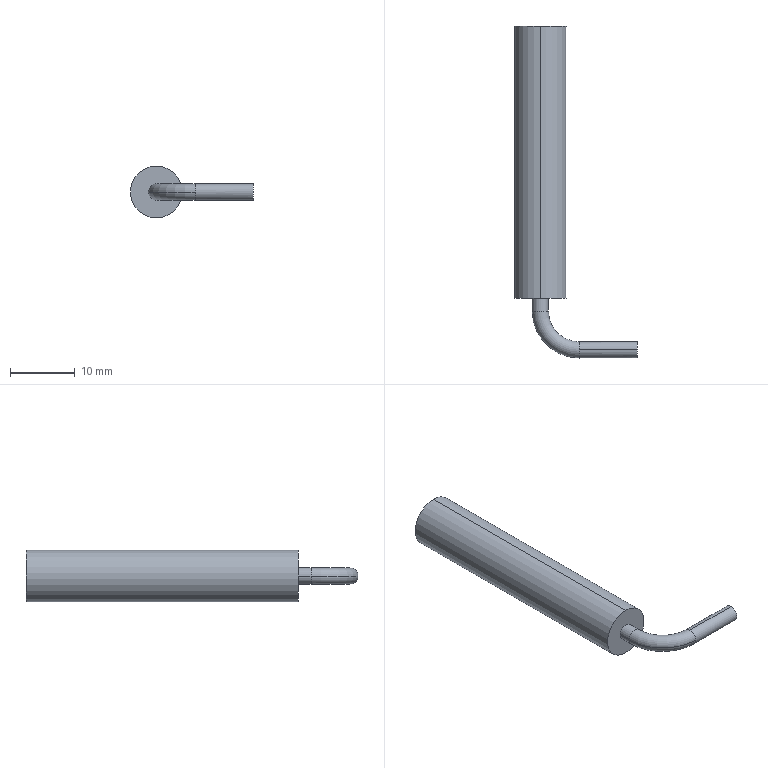Part | SolidWorks | features Extrusion 1, PLine 1, Sweep 1 | 1 solid | 12 faces | box 19 x 51.25 x 8 mm | volume 2211 mm3 | cylinder 6 | plane 4 | torus 2 | commonest cylinder face diameters 2.5 x4 8 x2
STEP:
#1=CARTESIAN_POINT('',(1.25,-2.,0.));
#2=VERTEX_POINT('',#1);
#3=CARTESIAN_POINT('',(-1.25,-2.,0.));
#4=VERTEX_POINT('',#3);
#5=CARTESIAN_POINT('',(0.,-2.,0.));
#6=DIRECTION('',(0.,-1.,0.));
#7=DIRECTION('',(0.,0.,-1.));
#8=AXIS2_PLACEMENT_3D('',#5,#6,#7);
#9=CIRCLE('',#8,1.25);
#10=EDGE_CURVE('',#2,#4,#9,.T.);
#11=ORIENTED_EDGE('',*,*,#10,.T.);
#12=CARTESIAN_POINT('',(6.,-9.25,0.));
#13=VERTEX_POINT('',#12);
#14=CARTESIAN_POINT('',(6.,-2.,0.));
#15=DIRECTION('',(0.,0.,1.));
#16=DIRECTION('',(1.,0.,0.));
#17=AXIS2_PLACEMENT_3D('',#14,#15,#16);
#18=CIRCLE('',#17,7.25);
#19=EDGE_CURVE('',#4,#13,#18,.T.);
#20=ORIENTED_EDGE('',*,*,#19,.T.);
#21=CARTESIAN_POINT('',(6.,-8.,1.25));
#22=VERTEX_POINT('',#21);
#23=CARTESIAN_POINT('',(6.,-8.,0.));
#24=DIRECTION('',(1.,0.,0.));
#25=DIRECTION('',(0.,0.,-1.));
#26=AXIS2_PLACEMENT_3D('',#23,#24,#25);
#27=CIRCLE('',#26,1.25);
#28=EDGE_CURVE('',#22,#13,#27,.T.);
#29=ORIENTED_EDGE('',*,*,#28,.F.);
#30=CARTESIAN_POINT('',(6.,-6.75,0.));
#31=VERTEX_POINT('',#30);
#32=CARTESIAN_POINT('',(6.,-8.,0.));
#33=DIRECTION('',(1.,0.,0.));
#34=DIRECTION('',(0.,0.,-1.));
#35=AXIS2_PLACEMENT_3D('',#32,#33,#34);
#36=CIRCLE('',#35,1.25);
#37=EDGE_CURVE('',#31,#22,#36,.T.);
#38=ORIENTED_EDGE('',*,*,#37,.F.);
#39=CARTESIAN_POINT('',(6.,-2.,0.));
#40=DIRECTION('',(0.,0.,1.));
#41=DIRECTION('',(1.,0.,0.));
#42=AXIS2_PLACEMENT_3D('',#39,#40,#41);
#43=CIRCLE('',#42,4.75);
#44=EDGE_CURVE('',#2,#31,#43,.T.);
#45=ORIENTED_EDGE('',*,*,#44,.F.);
#46=EDGE_LOOP('',(#11,#20,#29,#38,#45));
#47=FACE_OUTER_BOUND('',#46,.T.);
#48=CARTESIAN_POINT('',(6.,-2.,0.));
#49=DIRECTION('',(0.,0.,1.));
#50=DIRECTION('',(1.,0.,0.));
#51=AXIS2_PLACEMENT_3D('',#48,#49,#50);
#52=TOROIDAL_SURFACE('',#51,6.,1.25);
#53=ADVANCED_FACE('',(#47),#52,.T.);
#54=CARTESIAN_POINT('',(6.,-8.,-1.25));
#55=VERTEX_POINT('',#54);
#56=CARTESIAN_POINT('',(6.,-8.,0.));
#57=DIRECTION('',(1.,0.,0.));
#58=DIRECTION('',(0.,0.,-1.));
#59=AXIS2_PLACEMENT_3D('',#56,#57,#58);
#60=CIRCLE('',#59,1.25);
#61=EDGE_CURVE('',#55,#31,#60,.T.);
#62=ORIENTED_EDGE('',*,*,#61,.T.);
#63=ORIENTED_EDGE('',*,*,#37,.T.);
#64=CARTESIAN_POINT('',(15.,-8.,1.25));
#65=VERTEX_POINT('',#64);
#66=CARTESIAN_POINT('',(6.,-8.,1.25));
#67=DIRECTION('',(1.,0.,0.));
#68=VECTOR('',#67,1000.);
#69=LINE('',#66,#68);
#70=EDGE_CURVE('',#22,#65,#69,.T.);
#71=ORIENTED_EDGE('',*,*,#70,.T.);
#72=CARTESIAN_POINT('',(15.,-8.,-1.25));
#73=VERTEX_POINT('',#72);
#74=CARTESIAN_POINT('',(15.,-8.,0.));
#75=DIRECTION('',(1.,0.,0.));
#76=DIRECTION('',(0.,0.,-1.));
#77=AXIS2_PLACEMENT_3D('',#74,#75,#76);
#78=CIRCLE('',#77,1.25);
#79=EDGE_CURVE('',#73,#65,#78,.T.);
#80=ORIENTED_EDGE('',*,*,#79,.F.);
#81=CARTESIAN_POINT('',(6.,-8.,-1.25));
#82=DIRECTION('',(1.,0.,0.));
#83=VECTOR('',#82,1000.);
#84=LINE('',#81,#83);
#85=EDGE_CURVE('',#55,#73,#84,.T.);
#86=ORIENTED_EDGE('',*,*,#85,.F.);
#87=EDGE_LOOP('',(#62,#63,#71,#80,#86));
#88=FACE_OUTER_BOUND('',#87,.T.);
#89=CARTESIAN_POINT('',(6.,-8.,0.));
#90=DIRECTION('',(1.,0.,0.));
#91=DIRECTION('',(0.,0.,-1.));
#92=AXIS2_PLACEMENT_3D('',#89,#90,#91);
#93=CYLINDRICAL_SURFACE('',#92,1.25);
#94=ADVANCED_FACE('',(#88),#93,.T.);
#95=CARTESIAN_POINT('',(1.25,0.,0.));
#96=VERTEX_POINT('',#95);
#97=CARTESIAN_POINT('',(-1.25,0.,0.));
#98=VERTEX_POINT('',#97);
#99=CARTESIAN_POINT('',(0.,0.,0.));
#100=DIRECTION('',(0.,-1.,0.));
#101=DIRECTION('',(0.,0.,-1.));
#102=AXIS2_PLACEMENT_3D('',#99,#100,#101);
#103=CIRCLE('',#102,1.25);
#104=EDGE_CURVE('',#96,#98,#103,.T.);
#105=ORIENTED_EDGE('',*,*,#104,.T.);
#106=CARTESIAN_POINT('',(-1.25,0.,0.));
#107=DIRECTION('',(0.,-1.,0.));
#108=VECTOR('',#107,1000.);
#109=LINE('',#106,#108);
#110=EDGE_CURVE('',#98,#4,#109,.T.);
#111=ORIENTED_EDGE('',*,*,#110,.T.);
#112=ORIENTED_EDGE('',*,*,#10,.F.);
#113=CARTESIAN_POINT('',(1.25,0.,0.));
#114=DIRECTION('',(0.,-1.,0.));
#115=VECTOR('',#114,1000.);
#116=LINE('',#113,#115);
#117=EDGE_CURVE('',#96,#2,#116,.T.);
#118=ORIENTED_EDGE('',*,*,#117,.F.);
#119=EDGE_LOOP('',(#105,#111,#112,#118));
#120=FACE_OUTER_BOUND('',#119,.T.);
#121=CARTESIAN_POINT('',(0.,0.,0.));
#122=DIRECTION('',(0.,-1.,0.));
#123=DIRECTION('',(1.,0.,0.));
#124=AXIS2_PLACEMENT_3D('',#121,#122,#123);
#125=CYLINDRICAL_SURFACE('',#124,1.25);
#126=ADVANCED_FACE('',(#120),#125,.T.);
#127=CARTESIAN_POINT('',(0.,42.,4.));
#128=VERTEX_POINT('',#127);
#129=CARTESIAN_POINT('',(0.,42.,-4.));
#130=VERTEX_POINT('',#129);
#131=CARTESIAN_POINT('',(0.,42.,0.));
#132=DIRECTION('',(0.,1.,0.));
#133=DIRECTION('',(0.,0.,1.));
#134=AXIS2_PLACEMENT_3D('',#131,#132,#133);
#135=CIRCLE('',#134,4.);
#136=EDGE_CURVE('',#128,#130,#135,.T.);
#137=ORIENTED_EDGE('',*,*,#136,.F.);
#138=CARTESIAN_POINT('',(0.,0.,4.));
#139=VERTEX_POINT('',#138);
#140=CARTESIAN_POINT('',(0.,42.,4.));
#141=DIRECTION('',(0.,-1.,0.));
#142=VECTOR('',#141,1000.);
#143=LINE('',#140,#142);
#144=EDGE_CURVE('',#128,#139,#143,.T.);
#145=ORIENTED_EDGE('',*,*,#144,.T.);
#146=CARTESIAN_POINT('',(0.,0.,-4.));
#147=VERTEX_POINT('',#146);
#148=CARTESIAN_POINT('',(0.,0.,0.));
#149=DIRECTION('',(0.,1.,0.));
#150=DIRECTION('',(0.,0.,1.));
#151=AXIS2_PLACEMENT_3D('',#148,#149,#150);
#152=CIRCLE('',#151,4.);
#153=EDGE_CURVE('',#139,#147,#152,.T.);
#154=ORIENTED_EDGE('',*,*,#153,.T.);
#155=CARTESIAN_POINT('',(0.,42.,-4.));
#156=DIRECTION('',(0.,-1.,0.));
#157=VECTOR('',#156,1000.);
#158=LINE('',#155,#157);
#159=EDGE_CURVE('',#130,#147,#158,.T.);
#160=ORIENTED_EDGE('',*,*,#159,.F.);
#161=EDGE_LOOP('',(#137,#145,#154,#160));
#162=FACE_OUTER_BOUND('',#161,.T.);
#163=CARTESIAN_POINT('',(0.,42.,0.));
#164=DIRECTION('',(0.,-1.,0.));
#165=DIRECTION('',(0.,0.,-1.));
#166=AXIS2_PLACEMENT_3D('',#163,#164,#165);
#167=CYLINDRICAL_SURFACE('',#166,4.);
#168=ADVANCED_FACE('',(#162),#167,.T.);
#169=CARTESIAN_POINT('',(0.,42.,0.));
#170=DIRECTION('',(0.,1.,0.));
#171=DIRECTION('',(0.,0.,1.));
#172=AXIS2_PLACEMENT_3D('',#169,#170,#171);
#173=CIRCLE('',#172,4.);
#174=EDGE_CURVE('',#130,#128,#173,.T.);
#175=ORIENTED_EDGE('',*,*,#174,.T.);
#176=ORIENTED_EDGE('',*,*,#136,.T.);
#177=EDGE_LOOP('',(#175,#176));
#178=FACE_OUTER_BOUND('',#177,.T.);
#179=CARTESIAN_POINT('',(0.,42.,3.));
#180=VERTEX_POINT('',#179);
#181=CARTESIAN_POINT('',(0.,42.,-3.));
#182=VERTEX_POINT('',#181);
#183=CARTESIAN_POINT('',(0.,42.,0.));
#184=DIRECTION('',(0.,-1.,0.));
#185=DIRECTION('',(0.,0.,1.));
#186=AXIS2_PLACEMENT_3D('',#183,#184,#185);
#187=CIRCLE('',#186,3.);
#188=EDGE_CURVE('',#180,#182,#187,.T.);
#189=ORIENTED_EDGE('',*,*,#188,.T.);
#190=CARTESIAN_POINT('',(0.,42.,0.));
#191=DIRECTION('',(0.,-1.,0.));
#192=DIRECTION('',(0.,0.,1.));
#193=AXIS2_PLACEMENT_3D('',#190,#191,#192);
#194=CIRCLE('',#193,3.);
#195=EDGE_CURVE('',#182,#180,#194,.T.);
#196=ORIENTED_EDGE('',*,*,#195,.T.);
#197=EDGE_LOOP('',(#189,#196));
#198=FACE_BOUND('',#197,.T.);
#199=CARTESIAN_POINT('',(0.,42.,0.));
#200=DIRECTION('',(0.,1.,0.));
#201=DIRECTION('',(0.,0.,1.));
#202=AXIS2_PLACEMENT_3D('',#199,#200,#201);
#203=PLANE('',#202);
#204=ADVANCED_FACE('',(#178,#198),#203,.T.);
#205=ORIENTED_EDGE('',*,*,#144,.F.);
#206=ORIENTED_EDGE('',*,*,#174,.F.);
#207=ORIENTED_EDGE('',*,*,#159,.T.);
#208=CARTESIAN_POINT('',(0.,0.,0.));
#209=DIRECTION('',(0.,1.,0.));
#210=DIRECTION('',(0.,0.,1.));
#211=AXIS2_PLACEMENT_3D('',#208,#209,#210);
#212=CIRCLE('',#211,4.);
#213=EDGE_CURVE('',#147,#139,#212,.T.);
#214=ORIENTED_EDGE('',*,*,#213,.T.);
#215=EDGE_LOOP('',(#205,#206,#207,#214));
#216=FACE_OUTER_BOUND('',#215,.T.);
#217=CARTESIAN_POINT('',(0.,42.,0.));
#218=DIRECTION('',(0.,-1.,0.));
#219=DIRECTION('',(0.,0.,-1.));
#220=AXIS2_PLACEMENT_3D('',#217,#218,#219);
#221=CYLINDRICAL_SURFACE('',#220,4.);
#222=ADVANCED_FACE('',(#216),#221,.T.);
#223=ORIENTED_EDGE('',*,*,#188,.F.);
#224=ORIENTED_EDGE('',*,*,#195,.F.);
#225=EDGE_LOOP('',(#223,#224));
#226=FACE_OUTER_BOUND('',#225,.T.);
#227=CARTESIAN_POINT('',(0.,42.,0.));
#228=DIRECTION('',(0.,1.,0.));
#229=DIRECTION('',(0.,0.,1.));
#230=AXIS2_PLACEMENT_3D('',#227,#228,#229);
#231=PLANE('',#230);
#232=ADVANCED_FACE('',(#226),#231,.T.);
#233=ORIENTED_EDGE('',*,*,#104,.F.);
#234=CARTESIAN_POINT('',(0.,0.,0.));
#235=DIRECTION('',(0.,-1.,0.));
#236=DIRECTION('',(0.,0.,-1.));
#237=AXIS2_PLACEMENT_3D('',#234,#235,#236);
#238=CIRCLE('',#237,1.25);
#239=EDGE_CURVE('',#98,#96,#238,.T.);
#240=ORIENTED_EDGE('',*,*,#239,.F.);
#241=EDGE_LOOP('',(#233,#240));
#242=FACE_BOUND('',#241,.T.);
#243=ORIENTED_EDGE('',*,*,#213,.F.);
#244=ORIENTED_EDGE('',*,*,#153,.F.);
#245=EDGE_LOOP('',(#243,#244));
#246=FACE_OUTER_BOUND('',#245,.T.);
#247=CARTESIAN_POINT('',(0.,0.,0.));
#248=DIRECTION('',(0.,1.,0.));
#249=DIRECTION('',(0.,0.,1.));
#250=AXIS2_PLACEMENT_3D('',#247,#248,#249);
#251=PLANE('',#250);
#252=ADVANCED_FACE('',(#242,#246),#251,.F.);
#253=ORIENTED_EDGE('',*,*,#70,.F.);
#254=ORIENTED_EDGE('',*,*,#28,.T.);
#255=CARTESIAN_POINT('',(6.,-8.,0.));
#256=DIRECTION('',(1.,0.,0.));
#257=DIRECTION('',(0.,0.,-1.));
#258=AXIS2_PLACEMENT_3D('',#255,#256,#257);
#259=CIRCLE('',#258,1.25);
#260=EDGE_CURVE('',#13,#55,#259,.T.);
#261=ORIENTED_EDGE('',*,*,#260,.T.);
#262=ORIENTED_EDGE('',*,*,#85,.T.);
#263=CARTESIAN_POINT('',(15.,-8.,0.));
#264=DIRECTION('',(1.,0.,0.));
#265=DIRECTION('',(0.,0.,-1.));
#266=AXIS2_PLACEMENT_3D('',#263,#264,#265);
#267=CIRCLE('',#266,1.25);
#268=EDGE_CURVE('',#65,#73,#267,.T.);
#269=ORIENTED_EDGE('',*,*,#268,.F.);
#270=EDGE_LOOP('',(#253,#254,#261,#262,#269));
#271=FACE_OUTER_BOUND('',#270,.T.);
#272=CARTESIAN_POINT('',(6.,-8.,0.));
#273=DIRECTION('',(1.,0.,0.));
#274=DIRECTION('',(0.,0.,-1.));
#275=AXIS2_PLACEMENT_3D('',#272,#273,#274);
#276=CYLINDRICAL_SURFACE('',#275,1.25);
#277=ADVANCED_FACE('',(#271),#276,.T.);
#278=ORIENTED_EDGE('',*,*,#19,.F.);
#279=CARTESIAN_POINT('',(0.,-2.,0.));
#280=DIRECTION('',(0.,-1.,0.));
#281=DIRECTION('',(0.,0.,-1.));
#282=AXIS2_PLACEMENT_3D('',#279,#280,#281);
#283=CIRCLE('',#282,1.25);
#284=EDGE_CURVE('',#4,#2,#283,.T.);
#285=ORIENTED_EDGE('',*,*,#284,.T.);
#286=ORIENTED_EDGE('',*,*,#44,.T.);
#287=ORIENTED_EDGE('',*,*,#61,.F.);
#288=ORIENTED_EDGE('',*,*,#260,.F.);
#289=EDGE_LOOP('',(#278,#285,#286,#287,#288));
#290=FACE_OUTER_BOUND('',#289,.T.);
#291=CARTESIAN_POINT('',(6.,-2.,0.));
#292=DIRECTION('',(0.,0.,1.));
#293=DIRECTION('',(1.,0.,0.));
#294=AXIS2_PLACEMENT_3D('',#291,#292,#293);
#295=TOROIDAL_SURFACE('',#294,6.,1.25);
#296=ADVANCED_FACE('',(#290),#295,.T.);
#297=ORIENTED_EDGE('',*,*,#110,.F.);
#298=ORIENTED_EDGE('',*,*,#239,.T.);
#299=ORIENTED_EDGE('',*,*,#117,.T.);
#300=ORIENTED_EDGE('',*,*,#284,.F.);
#301=EDGE_LOOP('',(#297,#298,#299,#300));
#302=FACE_OUTER_BOUND('',#301,.T.);
#303=CARTESIAN_POINT('',(0.,0.,0.));
#304=DIRECTION('',(0.,-1.,0.));
#305=DIRECTION('',(1.,0.,0.));
#306=AXIS2_PLACEMENT_3D('',#303,#304,#305);
#307=CYLINDRICAL_SURFACE('',#306,1.25);
#308=ADVANCED_FACE('',(#302),#307,.T.);
#309=ORIENTED_EDGE('',*,*,#79,.T.);
#310=ORIENTED_EDGE('',*,*,#268,.T.);
#311=EDGE_LOOP('',(#309,#310));
#312=FACE_OUTER_BOUND('',#311,.T.);
#313=CARTESIAN_POINT('',(15.,-8.,0.));
#314=DIRECTION('',(1.,0.,0.));
#315=DIRECTION('',(0.,0.,-1.));
#316=AXIS2_PLACEMENT_3D('',#313,#314,#315);
#317=PLANE('',#316);
#318=ADVANCED_FACE('',(#312),#317,.T.);
#319=CLOSED_SHELL('',(#53,#94,#126,#168,#204,#222,#232,#252,#277,#296,#308,#318));
#320=MANIFOLD_SOLID_BREP('',#319);
#321=CARTESIAN_POINT('',(0.,0.,0.));
#322=DIRECTION('',(0.,0.,1.));
#323=DIRECTION('',(1.,0.,0.));
#324=AXIS2_PLACEMENT_3D('',#321,#322,#323);
#325=(LENGTH_UNIT()NAMED_UNIT(*)SI_UNIT(.MILLI.,.METRE.));
#326=UNCERTAINTY_MEASURE_WITH_UNIT(LENGTH_MEASURE(0.00001),#325,'','');
#327=(NAMED_UNIT(*)PLANE_ANGLE_UNIT()SI_UNIT($,.RADIAN.));
#328=(NAMED_UNIT(*)SI_UNIT($,.STERADIAN.)SOLID_ANGLE_UNIT());
#329=(GEOMETRIC_REPRESENTATION_CONTEXT(3)GLOBAL_UNCERTAINTY_ASSIGNED_CONTEXT((#326))GLOBAL_UNIT_ASSIGNED_CONTEXT((#325,#327,#328))REPRESENTATION_CONTEXT('',''));
#330=ADVANCED_BREP_SHAPE_REPRESENTATION('',(#320,#324),#329);